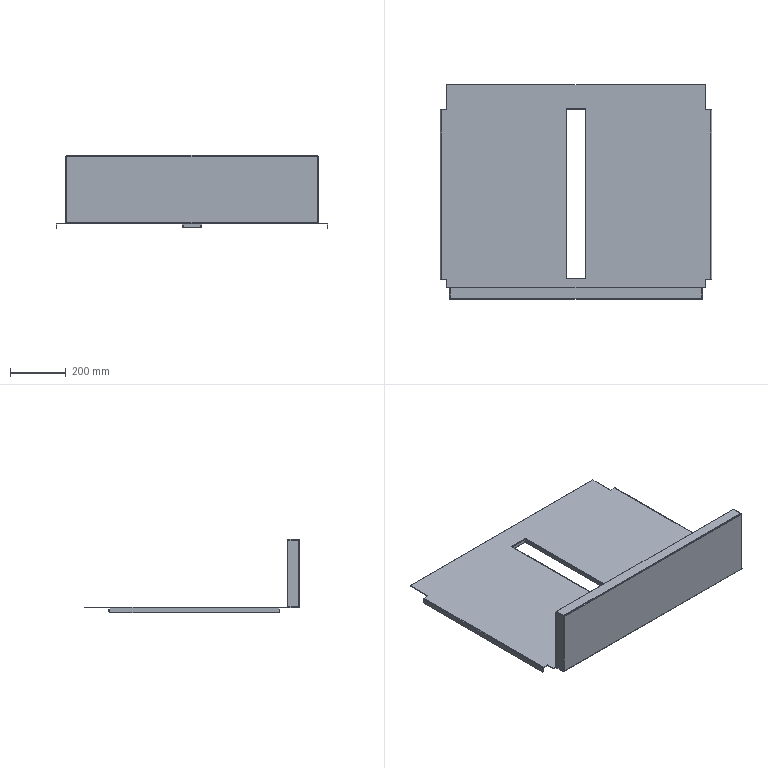Part | SolidWorks | features BaseBody 1 | 1 solid | 104 faces | box 973 x 767.4 x 263 mm | volume 2510755 mm3 | plane 72 | cylinder 20 | spline 12 | commonest cylinder face diameters 1 x10 6 x10